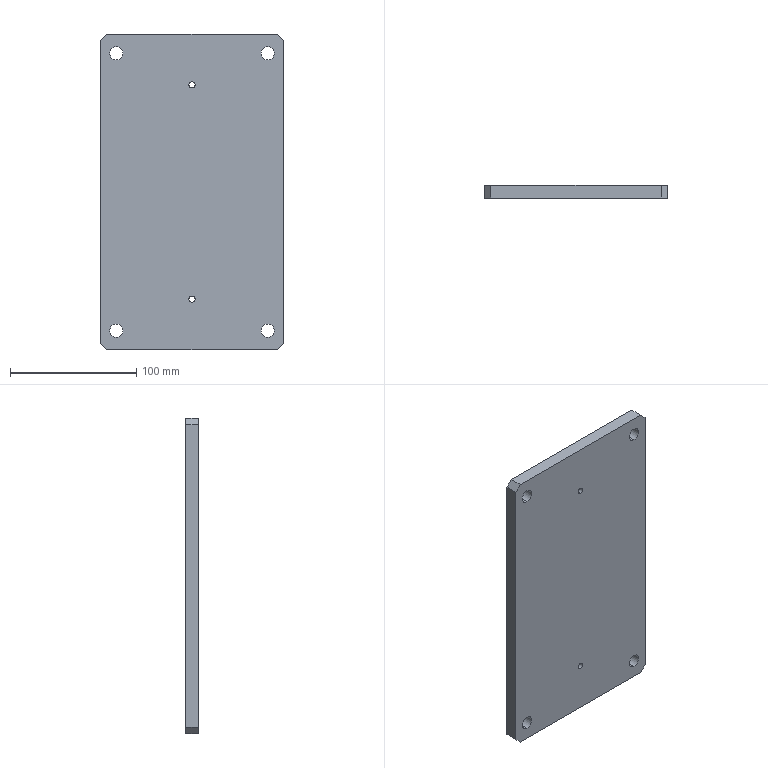Part | STEP file | PN_0031 | 1 solid | 22 faces | box 145 x 10 x 250 mm | volume 358144 mm3 | cylinder 12 | plane 10 | commonest cylinder face diameters 10.5 x8 5 x4